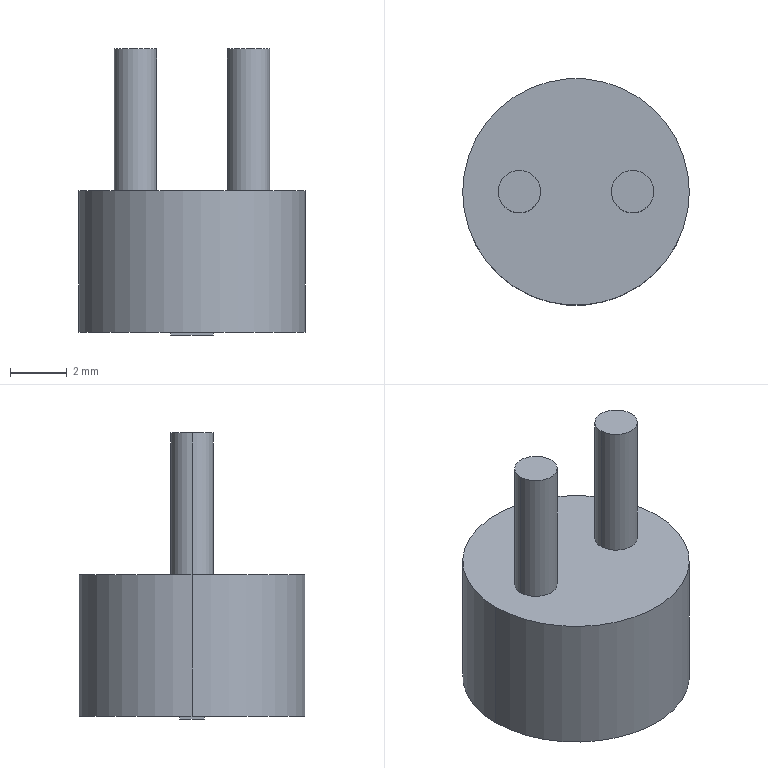Part | STEP file | 332 | 1 solid | 15 faces | box 8 x 8 x 10.1 mm | volume 269.13 mm3 | plane 9 | cylinder 6 | commonest cylinder face diameters 1.5 x4 8 x2
STEP:
#1=CARTESIAN_POINT('',(0.,0.,0.));
#2=DIRECTION('',(0.,0.,1.));
#3=DIRECTION('',(1.,0.,0.));
#4=AXIS2_PLACEMENT_3D('',#1,#2,#3);
#5=CARTESIAN_POINT('',(2.75,0.,10.));
#6=VERTEX_POINT('',#5);
#7=CARTESIAN_POINT('',(1.25,0.,10.));
#8=VERTEX_POINT('',#7);
#9=CARTESIAN_POINT('',(2.,0.,10.));
#10=DIRECTION('',(0.,0.,1.));
#11=DIRECTION('',(-1.,0.,0.));
#12=AXIS2_PLACEMENT_3D('',#9,#10,#11);
#13=CIRCLE('',#12,0.75);
#14=CARTESIAN_POINT('',(2.,0.,10.));
#15=DIRECTION('',(0.,0.,-1.));
#16=DIRECTION('',(-1.,0.,0.));
#17=AXIS2_PLACEMENT_3D('',#14,#15,#16);
#18=CYLINDRICAL_SURFACE('',#17,0.75);
#19=CARTESIAN_POINT('',(6.283,0.));
#20=DIRECTION('',(-1.,0.));
#21=VECTOR('',#20,1.);
#22=LINE('',#19,#21);
#23=(GEOMETRIC_REPRESENTATION_CONTEXT(2)PARAMETRIC_REPRESENTATION_CONTEXT()REPRESENTATION_CONTEXT('',''));
#24=DEFINITIONAL_REPRESENTATION('',(#22),#23);
#25=PCURVE('',#18,#24);
#26=CARTESIAN_POINT('',(2.,0.,10.));
#27=DIRECTION('',(0.,0.,-1.));
#28=DIRECTION('',(-1.,0.,0.));
#29=AXIS2_PLACEMENT_3D('',#26,#27,#28);
#30=PLANE('',#29);
#31=CARTESIAN_POINT('',(0.75,0.));
#32=CARTESIAN_POINT('',(0.75,-1.299));
#33=CARTESIAN_POINT('',(-0.375,-0.6495));
#34=CARTESIAN_POINT('',(-1.5,0.));
#35=CARTESIAN_POINT('',(-0.375,0.6495));
#36=CARTESIAN_POINT('',(0.75,1.299));
#37=CARTESIAN_POINT('',(0.75,0.));
#38=(BOUNDED_CURVE()B_SPLINE_CURVE(2,(#31,#32,#33,#34,#35,#36,#37),.UNSPECIFIED.,.T.,.F.)B_SPLINE_CURVE_WITH_KNOTS((1,2,2,2,2,1),(-2.094,0.,2.094,4.189,6.283,8.378),.UNSPECIFIED.)CURVE()GEOMETRIC_REPRESENTATION_ITEM()RATIONAL_B_SPLINE_CURVE((1.,0.5,1.,0.5,1.,0.5,1.))REPRESENTATION_ITEM(''));
#39=(GEOMETRIC_REPRESENTATION_CONTEXT(2)PARAMETRIC_REPRESENTATION_CONTEXT()REPRESENTATION_CONTEXT('',''));
#40=DEFINITIONAL_REPRESENTATION('',(#38),#39);
#41=PCURVE('',#30,#40);
#42=SURFACE_CURVE('',#13,(#25,#41),.PCURVE_S1.);
#43=EDGE_CURVE('',#6,#8,#42,.T.);
#44=ORIENTED_EDGE('',*,*,#43,.F.);
#45=CARTESIAN_POINT('',(2.75,0.,5.));
#46=VERTEX_POINT('',#45);
#47=CARTESIAN_POINT('',(2.75,0.,10.));
#48=DIRECTION('',(0.,0.,-1.));
#49=VECTOR('',#48,1.);
#50=LINE('',#47,#49);
#51=CARTESIAN_POINT('',(3.142,0.));
#52=DIRECTION('',(0.,1.));
#53=VECTOR('',#52,1.);
#54=LINE('',#51,#53);
#55=(GEOMETRIC_REPRESENTATION_CONTEXT(2)PARAMETRIC_REPRESENTATION_CONTEXT()REPRESENTATION_CONTEXT('',''));
#56=DEFINITIONAL_REPRESENTATION('',(#54),#55);
#57=PCURVE('',#18,#56);
#58=CARTESIAN_POINT('',(2.,0.,10.));
#59=DIRECTION('',(0.,0.,-1.));
#60=DIRECTION('',(-1.,0.,0.));
#61=AXIS2_PLACEMENT_3D('',#58,#59,#60);
#62=CYLINDRICAL_SURFACE('',#61,0.75);
#63=CARTESIAN_POINT('',(3.142,0.));
#64=DIRECTION('',(0.,1.));
#65=VECTOR('',#64,1.);
#66=LINE('',#63,#65);
#67=(GEOMETRIC_REPRESENTATION_CONTEXT(2)PARAMETRIC_REPRESENTATION_CONTEXT()REPRESENTATION_CONTEXT('',''));
#68=DEFINITIONAL_REPRESENTATION('',(#66),#67);
#69=PCURVE('',#62,#68);
#70=SURFACE_CURVE('',#50,(#57,#69),.PCURVE_S1.);
#71=EDGE_CURVE('',#6,#46,#70,.T.);
#72=ORIENTED_EDGE('',*,*,#71,.T.);
#73=CARTESIAN_POINT('',(1.25,0.,5.));
#74=VERTEX_POINT('',#73);
#75=CARTESIAN_POINT('',(2.,0.,5.));
#76=DIRECTION('',(0.,0.,1.));
#77=DIRECTION('',(-1.,0.,0.));
#78=AXIS2_PLACEMENT_3D('',#75,#76,#77);
#79=CIRCLE('',#78,0.75);
#80=CARTESIAN_POINT('',(6.283,5.));
#81=DIRECTION('',(-1.,0.));
#82=VECTOR('',#81,1.);
#83=LINE('',#80,#82);
#84=(GEOMETRIC_REPRESENTATION_CONTEXT(2)PARAMETRIC_REPRESENTATION_CONTEXT()REPRESENTATION_CONTEXT('',''));
#85=DEFINITIONAL_REPRESENTATION('',(#83),#84);
#86=PCURVE('',#18,#85);
#87=CARTESIAN_POINT('',(0.,0.,5.));
#88=DIRECTION('',(0.,0.,1.));
#89=DIRECTION('',(1.,0.,0.));
#90=AXIS2_PLACEMENT_3D('',#87,#88,#89);
#91=PLANE('',#90);
#92=CARTESIAN_POINT('',(2.,0.));
#93=DIRECTION('',(-1.,0.));
#94=AXIS2_PLACEMENT_2D('',#92,#93);
#95=CIRCLE('',#94,0.75);
#96=(GEOMETRIC_REPRESENTATION_CONTEXT(2)PARAMETRIC_REPRESENTATION_CONTEXT()REPRESENTATION_CONTEXT('',''));
#97=DEFINITIONAL_REPRESENTATION('',(#95),#96);
#98=PCURVE('',#91,#97);
#99=SURFACE_CURVE('',#79,(#86,#98),.PCURVE_S1.);
#100=EDGE_CURVE('',#46,#74,#99,.T.);
#101=ORIENTED_EDGE('',*,*,#100,.T.);
#102=CARTESIAN_POINT('',(1.25,0.,10.));
#103=DIRECTION('',(0.,0.,-1.));
#104=VECTOR('',#103,1.);
#105=LINE('',#102,#104);
#106=CARTESIAN_POINT('',(0.,0.));
#107=DIRECTION('',(0.,1.));
#108=VECTOR('',#107,1.);
#109=LINE('',#106,#108);
#110=(GEOMETRIC_REPRESENTATION_CONTEXT(2)PARAMETRIC_REPRESENTATION_CONTEXT()REPRESENTATION_CONTEXT('',''));
#111=DEFINITIONAL_REPRESENTATION('',(#109),#110);
#112=PCURVE('',#18,#111);
#113=CARTESIAN_POINT('',(6.283,0.));
#114=DIRECTION('',(0.,1.));
#115=VECTOR('',#114,1.);
#116=LINE('',#113,#115);
#117=(GEOMETRIC_REPRESENTATION_CONTEXT(2)PARAMETRIC_REPRESENTATION_CONTEXT()REPRESENTATION_CONTEXT('',''));
#118=DEFINITIONAL_REPRESENTATION('',(#116),#117);
#119=PCURVE('',#62,#118);
#120=SURFACE_CURVE('',#105,(#112,#119),.PCURVE_S1.);
#121=EDGE_CURVE('',#8,#74,#120,.T.);
#122=ORIENTED_EDGE('',*,*,#121,.F.);
#123=EDGE_LOOP('',(#44,#72,#101,#122));
#124=FACE_BOUND('',#123,.T.);
#125=ADVANCED_FACE('',(#124),#18,.T.);
#126=CARTESIAN_POINT('',(-1.25,0.,10.));
#127=VERTEX_POINT('',#126);
#128=CARTESIAN_POINT('',(-2.75,0.,10.));
#129=VERTEX_POINT('',#128);
#130=CARTESIAN_POINT('',(-2.,0.,10.));
#131=DIRECTION('',(0.,0.,1.));
#132=DIRECTION('',(1.,0.,0.));
#133=AXIS2_PLACEMENT_3D('',#130,#131,#132);
#134=CIRCLE('',#133,0.75);
#135=CARTESIAN_POINT('',(-2.,0.,10.));
#136=DIRECTION('',(0.,0.,-1.));
#137=DIRECTION('',(-1.,0.,0.));
#138=AXIS2_PLACEMENT_3D('',#135,#136,#137);
#139=CYLINDRICAL_SURFACE('',#138,0.75);
#140=CARTESIAN_POINT('',(3.142,0.));
#141=DIRECTION('',(-1.,0.));
#142=VECTOR('',#141,1.);
#143=LINE('',#140,#142);
#144=(GEOMETRIC_REPRESENTATION_CONTEXT(2)PARAMETRIC_REPRESENTATION_CONTEXT()REPRESENTATION_CONTEXT('',''));
#145=DEFINITIONAL_REPRESENTATION('',(#143),#144);
#146=PCURVE('',#139,#145);
#147=CARTESIAN_POINT('',(-2.,0.,10.));
#148=DIRECTION('',(0.,0.,1.));
#149=DIRECTION('',(1.,0.,0.));
#150=AXIS2_PLACEMENT_3D('',#147,#148,#149);
#151=PLANE('',#150);
#152=CARTESIAN_POINT('',(0.,0.));
#153=DIRECTION('',(1.,0.));
#154=AXIS2_PLACEMENT_2D('',#152,#153);
#155=CIRCLE('',#154,0.75);
#156=(GEOMETRIC_REPRESENTATION_CONTEXT(2)PARAMETRIC_REPRESENTATION_CONTEXT()REPRESENTATION_CONTEXT('',''));
#157=DEFINITIONAL_REPRESENTATION('',(#155),#156);
#158=PCURVE('',#151,#157);
#159=SURFACE_CURVE('',#134,(#146,#158),.PCURVE_S1.);
#160=EDGE_CURVE('',#127,#129,#159,.T.);
#161=ORIENTED_EDGE('',*,*,#160,.F.);
#162=CARTESIAN_POINT('',(-1.25,0.,5.));
#163=VERTEX_POINT('',#162);
#164=CARTESIAN_POINT('',(-1.25,0.,10.));
#165=DIRECTION('',(0.,0.,-1.));
#166=VECTOR('',#165,1.);
#167=LINE('',#164,#166);
#168=CARTESIAN_POINT('',(3.142,0.));
#169=DIRECTION('',(0.,1.));
#170=VECTOR('',#169,1.);
#171=LINE('',#168,#170);
#172=(GEOMETRIC_REPRESENTATION_CONTEXT(2)PARAMETRIC_REPRESENTATION_CONTEXT()REPRESENTATION_CONTEXT('',''));
#173=DEFINITIONAL_REPRESENTATION('',(#171),#172);
#174=PCURVE('',#139,#173);
#175=CARTESIAN_POINT('',(-2.,0.,10.));
#176=DIRECTION('',(0.,0.,-1.));
#177=DIRECTION('',(-1.,0.,0.));
#178=AXIS2_PLACEMENT_3D('',#175,#176,#177);
#179=CYLINDRICAL_SURFACE('',#178,0.75);
#180=CARTESIAN_POINT('',(3.142,0.));
#181=DIRECTION('',(0.,1.));
#182=VECTOR('',#181,1.);
#183=LINE('',#180,#182);
#184=(GEOMETRIC_REPRESENTATION_CONTEXT(2)PARAMETRIC_REPRESENTATION_CONTEXT()REPRESENTATION_CONTEXT('',''));
#185=DEFINITIONAL_REPRESENTATION('',(#183),#184);
#186=PCURVE('',#179,#185);
#187=SURFACE_CURVE('',#167,(#174,#186),.PCURVE_S1.);
#188=EDGE_CURVE('',#127,#163,#187,.T.);
#189=ORIENTED_EDGE('',*,*,#188,.T.);
#190=CARTESIAN_POINT('',(-2.75,0.,5.));
#191=VERTEX_POINT('',#190);
#192=CARTESIAN_POINT('',(-2.,0.,5.));
#193=DIRECTION('',(0.,0.,1.));
#194=DIRECTION('',(1.,0.,0.));
#195=AXIS2_PLACEMENT_3D('',#192,#193,#194);
#196=CIRCLE('',#195,0.75);
#197=CARTESIAN_POINT('',(3.142,5.));
#198=DIRECTION('',(-1.,0.));
#199=VECTOR('',#198,1.);
#200=LINE('',#197,#199);
#201=(GEOMETRIC_REPRESENTATION_CONTEXT(2)PARAMETRIC_REPRESENTATION_CONTEXT()REPRESENTATION_CONTEXT('',''));
#202=DEFINITIONAL_REPRESENTATION('',(#200),#201);
#203=PCURVE('',#139,#202);
#204=CARTESIAN_POINT('',(-2.,0.));
#205=DIRECTION('',(1.,0.));
#206=AXIS2_PLACEMENT_2D('',#204,#205);
#207=CIRCLE('',#206,0.75);
#208=(GEOMETRIC_REPRESENTATION_CONTEXT(2)PARAMETRIC_REPRESENTATION_CONTEXT()REPRESENTATION_CONTEXT('',''));
#209=DEFINITIONAL_REPRESENTATION('',(#207),#208);
#210=PCURVE('',#91,#209);
#211=SURFACE_CURVE('',#196,(#203,#210),.PCURVE_S1.);
#212=EDGE_CURVE('',#163,#191,#211,.T.);
#213=ORIENTED_EDGE('',*,*,#212,.T.);
#214=CARTESIAN_POINT('',(-2.75,0.,10.));
#215=DIRECTION('',(0.,0.,-1.));
#216=VECTOR('',#215,1.);
#217=LINE('',#214,#216);
#218=CARTESIAN_POINT('',(0.,0.));
#219=DIRECTION('',(0.,1.));
#220=VECTOR('',#219,1.);
#221=LINE('',#218,#220);
#222=(GEOMETRIC_REPRESENTATION_CONTEXT(2)PARAMETRIC_REPRESENTATION_CONTEXT()REPRESENTATION_CONTEXT('',''));
#223=DEFINITIONAL_REPRESENTATION('',(#221),#222);
#224=PCURVE('',#139,#223);
#225=CARTESIAN_POINT('',(6.283,0.));
#226=DIRECTION('',(0.,1.));
#227=VECTOR('',#226,1.);
#228=LINE('',#225,#227);
#229=(GEOMETRIC_REPRESENTATION_CONTEXT(2)PARAMETRIC_REPRESENTATION_CONTEXT()REPRESENTATION_CONTEXT('',''));
#230=DEFINITIONAL_REPRESENTATION('',(#228),#229);
#231=PCURVE('',#179,#230);
#232=SURFACE_CURVE('',#217,(#224,#231),.PCURVE_S1.);
#233=EDGE_CURVE('',#129,#191,#232,.T.);
#234=ORIENTED_EDGE('',*,*,#233,.F.);
#235=EDGE_LOOP('',(#161,#189,#213,#234));
#236=FACE_BOUND('',#235,.T.);
#237=ADVANCED_FACE('',(#236),#139,.T.);
#238=CARTESIAN_POINT('',(4.,0.,5.));
#239=VERTEX_POINT('',#238);
#240=CARTESIAN_POINT('',(-4.,0.,5.));
#241=VERTEX_POINT('',#240);
#242=CARTESIAN_POINT('',(0.,0.,5.));
#243=DIRECTION('',(0.,0.,1.));
#244=DIRECTION('',(1.,0.,0.));
#245=AXIS2_PLACEMENT_3D('',#242,#243,#244);
#246=CIRCLE('',#245,4.);
#247=CARTESIAN_POINT('',(0.,0.,5.));
#248=DIRECTION('',(0.,0.,-1.));
#249=DIRECTION('',(-1.,0.,0.));
#250=AXIS2_PLACEMENT_3D('',#247,#248,#249);
#251=CYLINDRICAL_SURFACE('',#250,4.);
#252=CARTESIAN_POINT('',(3.142,0.));
#253=DIRECTION('',(-1.,0.));
#254=VECTOR('',#253,1.);
#255=LINE('',#252,#254);
#256=(GEOMETRIC_REPRESENTATION_CONTEXT(2)PARAMETRIC_REPRESENTATION_CONTEXT()REPRESENTATION_CONTEXT('',''));
#257=DEFINITIONAL_REPRESENTATION('',(#255),#256);
#258=PCURVE('',#251,#257);
#259=CARTESIAN_POINT('',(0.,0.));
#260=DIRECTION('',(1.,0.));
#261=AXIS2_PLACEMENT_2D('',#259,#260);
#262=CIRCLE('',#261,4.);
#263=(GEOMETRIC_REPRESENTATION_CONTEXT(2)PARAMETRIC_REPRESENTATION_CONTEXT()REPRESENTATION_CONTEXT('',''));
#264=DEFINITIONAL_REPRESENTATION('',(#262),#263);
#265=PCURVE('',#91,#264);
#266=SURFACE_CURVE('',#246,(#258,#265),.PCURVE_S1.);
#267=EDGE_CURVE('',#239,#241,#266,.T.);
#268=ORIENTED_EDGE('',*,*,#267,.F.);
#269=CARTESIAN_POINT('',(4.,0.,0.));
#270=VERTEX_POINT('',#269);
#271=CARTESIAN_POINT('',(4.,0.,5.));
#272=DIRECTION('',(0.,0.,-1.));
#273=VECTOR('',#272,1.);
#274=LINE('',#271,#273);
#275=CARTESIAN_POINT('',(3.142,0.));
#276=DIRECTION('',(0.,1.));
#277=VECTOR('',#276,1.);
#278=LINE('',#275,#277);
#279=(GEOMETRIC_REPRESENTATION_CONTEXT(2)PARAMETRIC_REPRESENTATION_CONTEXT()REPRESENTATION_CONTEXT('',''));
#280=DEFINITIONAL_REPRESENTATION('',(#278),#279);
#281=PCURVE('',#251,#280);
#282=CARTESIAN_POINT('',(0.,0.,5.));
#283=DIRECTION('',(0.,0.,-1.));
#284=DIRECTION('',(-1.,0.,0.));
#285=AXIS2_PLACEMENT_3D('',#282,#283,#284);
#286=CYLINDRICAL_SURFACE('',#285,4.);
#287=CARTESIAN_POINT('',(3.142,0.));
#288=DIRECTION('',(0.,1.));
#289=VECTOR('',#288,1.);
#290=LINE('',#287,#289);
#291=(GEOMETRIC_REPRESENTATION_CONTEXT(2)PARAMETRIC_REPRESENTATION_CONTEXT()REPRESENTATION_CONTEXT('',''));
#292=DEFINITIONAL_REPRESENTATION('',(#290),#291);
#293=PCURVE('',#286,#292);
#294=SURFACE_CURVE('',#274,(#281,#293),.PCURVE_S1.);
#295=EDGE_CURVE('',#239,#270,#294,.T.);
#296=ORIENTED_EDGE('',*,*,#295,.T.);
#297=CARTESIAN_POINT('',(-4.,0.,0.));
#298=VERTEX_POINT('',#297);
#299=CARTESIAN_POINT('',(0.,0.,0.));
#300=DIRECTION('',(0.,0.,1.));
#301=DIRECTION('',(1.,0.,0.));
#302=AXIS2_PLACEMENT_3D('',#299,#300,#301);
#303=CIRCLE('',#302,4.);
#304=CARTESIAN_POINT('',(3.142,5.));
#305=DIRECTION('',(-1.,0.));
#306=VECTOR('',#305,1.);
#307=LINE('',#304,#306);
#308=(GEOMETRIC_REPRESENTATION_CONTEXT(2)PARAMETRIC_REPRESENTATION_CONTEXT()REPRESENTATION_CONTEXT('',''));
#309=DEFINITIONAL_REPRESENTATION('',(#307),#308);
#310=PCURVE('',#251,#309);
#311=CARTESIAN_POINT('',(0.,0.,0.));
#312=DIRECTION('',(0.,0.,1.));
#313=DIRECTION('',(1.,0.,0.));
#314=AXIS2_PLACEMENT_3D('',#311,#312,#313);
#315=PLANE('',#314);
#316=CARTESIAN_POINT('',(0.,0.));
#317=DIRECTION('',(1.,0.));
#318=AXIS2_PLACEMENT_2D('',#316,#317);
#319=CIRCLE('',#318,4.);
#320=(GEOMETRIC_REPRESENTATION_CONTEXT(2)PARAMETRIC_REPRESENTATION_CONTEXT()REPRESENTATION_CONTEXT('',''));
#321=DEFINITIONAL_REPRESENTATION('',(#319),#320);
#322=PCURVE('',#315,#321);
#323=SURFACE_CURVE('',#303,(#310,#322),.PCURVE_S1.);
#324=EDGE_CURVE('',#270,#298,#323,.T.);
#325=ORIENTED_EDGE('',*,*,#324,.T.);
#326=CARTESIAN_POINT('',(-4.,0.,5.));
#327=DIRECTION('',(0.,0.,-1.));
#328=VECTOR('',#327,1.);
#329=LINE('',#326,#328);
#330=CARTESIAN_POINT('',(0.,0.));
#331=DIRECTION('',(0.,1.));
#332=VECTOR('',#331,1.);
#333=LINE('',#330,#332);
#334=(GEOMETRIC_REPRESENTATION_CONTEXT(2)PARAMETRIC_REPRESENTATION_CONTEXT()REPRESENTATION_CONTEXT('',''));
#335=DEFINITIONAL_REPRESENTATION('',(#333),#334);
#336=PCURVE('',#251,#335);
#337=CARTESIAN_POINT('',(6.283,0.));
#338=DIRECTION('',(0.,1.));
#339=VECTOR('',#338,1.);
#340=LINE('',#337,#339);
#341=(GEOMETRIC_REPRESENTATION_CONTEXT(2)PARAMETRIC_REPRESENTATION_CONTEXT()REPRESENTATION_CONTEXT('',''));
#342=DEFINITIONAL_REPRESENTATION('',(#340),#341);
#343=PCURVE('',#286,#342);
#344=SURFACE_CURVE('',#329,(#336,#343),.PCURVE_S1.);
#345=EDGE_CURVE('',#241,#298,#344,.T.);
#346=ORIENTED_EDGE('',*,*,#345,.F.);
#347=EDGE_LOOP('',(#268,#296,#325,#346));
#348=FACE_BOUND('',#347,.T.);
#349=ADVANCED_FACE('',(#348),#251,.T.);
#350=CARTESIAN_POINT('',(0.,0.,0.));
#351=DIRECTION('',(0.,0.,1.));
#352=DIRECTION('',(1.,0.,0.));
#353=AXIS2_PLACEMENT_3D('',#350,#351,#352);
#354=CIRCLE('',#353,4.);
#355=CARTESIAN_POINT('',(0.,0.));
#356=DIRECTION('',(1.,0.));
#357=AXIS2_PLACEMENT_2D('',#355,#356);
#358=CIRCLE('',#357,4.);
#359=(GEOMETRIC_REPRESENTATION_CONTEXT(2)PARAMETRIC_REPRESENTATION_CONTEXT()REPRESENTATION_CONTEXT('',''));
#360=DEFINITIONAL_REPRESENTATION('',(#358),#359);
#361=PCURVE('',#315,#360);
#362=CARTESIAN_POINT('',(9.425,5.));
#363=DIRECTION('',(-1.,0.));
#364=VECTOR('',#363,1.);
#365=LINE('',#362,#364);
#366=(GEOMETRIC_REPRESENTATION_CONTEXT(2)PARAMETRIC_REPRESENTATION_CONTEXT()REPRESENTATION_CONTEXT('',''));
#367=DEFINITIONAL_REPRESENTATION('',(#365),#366);
#368=PCURVE('',#286,#367);
#369=SURFACE_CURVE('',#354,(#361,#368),.PCURVE_S1.);
#370=EDGE_CURVE('',#298,#270,#369,.T.);
#371=ORIENTED_EDGE('',*,*,#370,.F.);
#372=ORIENTED_EDGE('',*,*,#324,.F.);
#373=EDGE_LOOP('',(#371,#372));
#374=FACE_BOUND('',#373,.T.);
#375=CARTESIAN_POINT('',(0.7479,0.4396,0.));
#376=VERTEX_POINT('',#375);
#377=CARTESIAN_POINT('',(0.7479,-0.4396,0.));
#378=VERTEX_POINT('',#377);
#379=CARTESIAN_POINT('',(0.7479,0.4396,0.));
#380=DIRECTION('',(0.,-1.,0.));
#381=VECTOR('',#380,1.);
#382=LINE('',#379,#381);
#383=CARTESIAN_POINT('',(0.7479,0.4396));
#384=DIRECTION('',(0.,-1.));
#385=VECTOR('',#384,1.);
#386=LINE('',#383,#385);
#387=(GEOMETRIC_REPRESENTATION_CONTEXT(2)PARAMETRIC_REPRESENTATION_CONTEXT()REPRESENTATION_CONTEXT('',''));
#388=DEFINITIONAL_REPRESENTATION('',(#386),#387);
#389=PCURVE('',#315,#388);
#390=CARTESIAN_POINT('',(0.7479,0.4396,-0.1));
#391=DIRECTION('',(-1.,0.,0.));
#392=DIRECTION('',(0.,0.,1.));
#393=AXIS2_PLACEMENT_3D('',#390,#391,#392);
#394=PLANE('',#393);
#395=CARTESIAN_POINT('',(0.1,0.));
#396=DIRECTION('',(0.,-1.));
#397=VECTOR('',#396,1.);
#398=LINE('',#395,#397);
#399=(GEOMETRIC_REPRESENTATION_CONTEXT(2)PARAMETRIC_REPRESENTATION_CONTEXT()REPRESENTATION_CONTEXT('',''));
#400=DEFINITIONAL_REPRESENTATION('',(#398),#399);
#401=PCURVE('',#394,#400);
#402=SURFACE_CURVE('',#382,(#389,#401),.PCURVE_S1.);
#403=EDGE_CURVE('',#376,#378,#402,.T.);
#404=ORIENTED_EDGE('',*,*,#403,.F.);
#405=CARTESIAN_POINT('',(-0.7479,0.4396,0.));
#406=VERTEX_POINT('',#405);
#407=CARTESIAN_POINT('',(-0.7479,0.4396,0.));
#408=DIRECTION('',(1.,0.,0.));
#409=VECTOR('',#408,1.);
#410=LINE('',#407,#409);
#411=CARTESIAN_POINT('',(-0.7479,0.4396));
#412=DIRECTION('',(1.,0.));
#413=VECTOR('',#412,1.);
#414=LINE('',#411,#413);
#415=(GEOMETRIC_REPRESENTATION_CONTEXT(2)PARAMETRIC_REPRESENTATION_CONTEXT()REPRESENTATION_CONTEXT('',''));
#416=DEFINITIONAL_REPRESENTATION('',(#414),#415);
#417=PCURVE('',#315,#416);
#418=CARTESIAN_POINT('',(-0.7479,0.4396,-0.1));
#419=DIRECTION('',(0.,-1.,0.));
#420=DIRECTION('',(0.,0.,-1.));
#421=AXIS2_PLACEMENT_3D('',#418,#419,#420);
#422=PLANE('',#421);
#423=CARTESIAN_POINT('',(-0.1,0.));
#424=DIRECTION('',(0.,1.));
#425=VECTOR('',#424,1.);
#426=LINE('',#423,#425);
#427=(GEOMETRIC_REPRESENTATION_CONTEXT(2)PARAMETRIC_REPRESENTATION_CONTEXT()REPRESENTATION_CONTEXT('',''));
#428=DEFINITIONAL_REPRESENTATION('',(#426),#427);
#429=PCURVE('',#422,#428);
#430=SURFACE_CURVE('',#410,(#417,#429),.PCURVE_S1.);
#431=EDGE_CURVE('',#406,#376,#430,.T.);
#432=ORIENTED_EDGE('',*,*,#431,.F.);
#433=CARTESIAN_POINT('',(-0.7479,-0.4396,0.));
#434=VERTEX_POINT('',#433);
#435=CARTESIAN_POINT('',(-0.7479,0.4396,0.));
#436=DIRECTION('',(0.,1.,0.));
#437=VECTOR('',#436,1.);
#438=LINE('',#435,#437);
#439=CARTESIAN_POINT('',(-0.7479,0.4396));
#440=DIRECTION('',(0.,1.));
#441=VECTOR('',#440,1.);
#442=LINE('',#439,#441);
#443=(GEOMETRIC_REPRESENTATION_CONTEXT(2)PARAMETRIC_REPRESENTATION_CONTEXT()REPRESENTATION_CONTEXT('',''));
#444=DEFINITIONAL_REPRESENTATION('',(#442),#443);
#445=PCURVE('',#315,#444);
#446=CARTESIAN_POINT('',(-0.7479,0.4396,-0.1));
#447=DIRECTION('',(1.,0.,0.));
#448=DIRECTION('',(0.,0.,-1.));
#449=AXIS2_PLACEMENT_3D('',#446,#447,#448);
#450=PLANE('',#449);
#451=CARTESIAN_POINT('',(-0.1,0.));
#452=DIRECTION('',(0.,1.));
#453=VECTOR('',#452,1.);
#454=LINE('',#451,#453);
#455=(GEOMETRIC_REPRESENTATION_CONTEXT(2)PARAMETRIC_REPRESENTATION_CONTEXT()REPRESENTATION_CONTEXT('',''));
#456=DEFINITIONAL_REPRESENTATION('',(#454),#455);
#457=PCURVE('',#450,#456);
#458=SURFACE_CURVE('',#438,(#445,#457),.PCURVE_S1.);
#459=EDGE_CURVE('',#434,#406,#458,.T.);
#460=ORIENTED_EDGE('',*,*,#459,.F.);
#461=CARTESIAN_POINT('',(-0.7479,-0.4396,0.));
#462=DIRECTION('',(-1.,0.,0.));
#463=VECTOR('',#462,1.);
#464=LINE('',#461,#463);
#465=CARTESIAN_POINT('',(-0.7479,-0.4396));
#466=DIRECTION('',(-1.,0.));
#467=VECTOR('',#466,1.);
#468=LINE('',#465,#467);
#469=(GEOMETRIC_REPRESENTATION_CONTEXT(2)PARAMETRIC_REPRESENTATION_CONTEXT()REPRESENTATION_CONTEXT('',''));
#470=DEFINITIONAL_REPRESENTATION('',(#468),#469);
#471=PCURVE('',#315,#470);
#472=CARTESIAN_POINT('',(-0.7479,-0.4396,-0.1));
#473=DIRECTION('',(0.,1.,0.));
#474=DIRECTION('',(0.,0.,1.));
#475=AXIS2_PLACEMENT_3D('',#472,#473,#474);
#476=PLANE('',#475);
#477=CARTESIAN_POINT('',(0.1,0.));
#478=DIRECTION('',(0.,-1.));
#479=VECTOR('',#478,1.);
#480=LINE('',#477,#479);
#481=(GEOMETRIC_REPRESENTATION_CONTEXT(2)PARAMETRIC_REPRESENTATION_CONTEXT()REPRESENTATION_CONTEXT('',''));
#482=DEFINITIONAL_REPRESENTATION('',(#480),#481);
#483=PCURVE('',#476,#482);
#484=SURFACE_CURVE('',#464,(#471,#483),.PCURVE_S1.);
#485=EDGE_CURVE('',#378,#434,#484,.T.);
#486=ORIENTED_EDGE('',*,*,#485,.F.);
#487=EDGE_LOOP('',(#404,#432,#460,#486));
#488=FACE_BOUND('',#487,.T.);
#489=ADVANCED_FACE('',(#374,#488),#315,.F.);
#490=CARTESIAN_POINT('',(-2.,0.,5.));
#491=DIRECTION('',(0.,0.,1.));
#492=DIRECTION('',(1.,0.,0.));
#493=AXIS2_PLACEMENT_3D('',#490,#491,#492);
#494=CIRCLE('',#493,0.75);
#495=CARTESIAN_POINT('',(-2.,0.));
#496=DIRECTION('',(1.,0.));
#497=AXIS2_PLACEMENT_2D('',#495,#496);
#498=CIRCLE('',#497,0.75);
#499=(GEOMETRIC_REPRESENTATION_CONTEXT(2)PARAMETRIC_REPRESENTATION_CONTEXT()REPRESENTATION_CONTEXT('',''));
#500=DEFINITIONAL_REPRESENTATION('',(#498),#499);
#501=PCURVE('',#91,#500);
#502=CARTESIAN_POINT('',(9.425,5.));
#503=DIRECTION('',(-1.,0.));
#504=VECTOR('',#503,1.);
#505=LINE('',#502,#504);
#506=(GEOMETRIC_REPRESENTATION_CONTEXT(2)PARAMETRIC_REPRESENTATION_CONTEXT()REPRESENTATION_CONTEXT('',''));
#507=DEFINITIONAL_REPRESENTATION('',(#505),#506);
#508=PCURVE('',#179,#507);
#509=SURFACE_CURVE('',#494,(#501,#508),.PCURVE_S1.);
#510=EDGE_CURVE('',#191,#163,#509,.T.);
#511=ORIENTED_EDGE('',*,*,#510,.F.);
#512=ORIENTED_EDGE('',*,*,#212,.F.);
#513=EDGE_LOOP('',(#511,#512));
#514=FACE_BOUND('',#513,.T.);
#515=CARTESIAN_POINT('',(0.,0.,5.));
#516=DIRECTION('',(0.,0.,1.));
#517=DIRECTION('',(1.,0.,0.));
#518=AXIS2_PLACEMENT_3D('',#515,#516,#517);
#519=CIRCLE('',#518,4.);
#520=CARTESIAN_POINT('',(0.,0.));
#521=DIRECTION('',(1.,0.));
#522=AXIS2_PLACEMENT_2D('',#520,#521);
#523=CIRCLE('',#522,4.);
#524=(GEOMETRIC_REPRESENTATION_CONTEXT(2)PARAMETRIC_REPRESENTATION_CONTEXT()REPRESENTATION_CONTEXT('',''));
#525=DEFINITIONAL_REPRESENTATION('',(#523),#524);
#526=PCURVE('',#91,#525);
#527=CARTESIAN_POINT('',(9.425,0.));
#528=DIRECTION('',(-1.,0.));
#529=VECTOR('',#528,1.);
#530=LINE('',#527,#529);
#531=(GEOMETRIC_REPRESENTATION_CONTEXT(2)PARAMETRIC_REPRESENTATION_CONTEXT()REPRESENTATION_CONTEXT('',''));
#532=DEFINITIONAL_REPRESENTATION('',(#530),#531);
#533=PCURVE('',#286,#532);
#534=SURFACE_CURVE('',#519,(#526,#533),.PCURVE_S1.);
#535=EDGE_CURVE('',#241,#239,#534,.T.);
#536=ORIENTED_EDGE('',*,*,#535,.T.);
#537=ORIENTED_EDGE('',*,*,#267,.T.);
#538=EDGE_LOOP('',(#536,#537));
#539=FACE_BOUND('',#538,.T.);
#540=CARTESIAN_POINT('',(2.,0.,5.));
#541=DIRECTION('',(0.,0.,1.));
#542=DIRECTION('',(-1.,0.,0.));
#543=AXIS2_PLACEMENT_3D('',#540,#541,#542);
#544=CIRCLE('',#543,0.75);
#545=CARTESIAN_POINT('',(2.,0.));
#546=DIRECTION('',(-1.,0.));
#547=AXIS2_PLACEMENT_2D('',#545,#546);
#548=CIRCLE('',#547,0.75);
#549=(GEOMETRIC_REPRESENTATION_CONTEXT(2)PARAMETRIC_REPRESENTATION_CONTEXT()REPRESENTATION_CONTEXT('',''));
#550=DEFINITIONAL_REPRESENTATION('',(#548),#549);
#551=PCURVE('',#91,#550);
#552=CARTESIAN_POINT('',(6.283,5.));
#553=DIRECTION('',(-1.,0.));
#554=VECTOR('',#553,1.);
#555=LINE('',#552,#554);
#556=(GEOMETRIC_REPRESENTATION_CONTEXT(2)PARAMETRIC_REPRESENTATION_CONTEXT()REPRESENTATION_CONTEXT('',''));
#557=DEFINITIONAL_REPRESENTATION('',(#555),#556);
#558=PCURVE('',#62,#557);
#559=SURFACE_CURVE('',#544,(#551,#558),.PCURVE_S1.);
#560=EDGE_CURVE('',#74,#46,#559,.T.);
#561=ORIENTED_EDGE('',*,*,#560,.F.);
#562=ORIENTED_EDGE('',*,*,#100,.F.);
#563=EDGE_LOOP('',(#561,#562));
#564=FACE_BOUND('',#563,.T.);
#565=ADVANCED_FACE('',(#514,#539,#564),#91,.T.);
#566=ORIENTED_EDGE('',*,*,#295,.F.);
#567=ORIENTED_EDGE('',*,*,#535,.F.);
#568=ORIENTED_EDGE('',*,*,#345,.T.);
#569=ORIENTED_EDGE('',*,*,#370,.T.);
#570=EDGE_LOOP('',(#566,#567,#568,#569));
#571=FACE_BOUND('',#570,.T.);
#572=ADVANCED_FACE('',(#571),#286,.T.);
#573=ORIENTED_EDGE('',*,*,#188,.F.);
#574=CARTESIAN_POINT('',(-2.,0.,10.));
#575=DIRECTION('',(0.,0.,1.));
#576=DIRECTION('',(1.,0.,0.));
#577=AXIS2_PLACEMENT_3D('',#574,#575,#576);
#578=CIRCLE('',#577,0.75);
#579=CARTESIAN_POINT('',(9.425,0.));
#580=DIRECTION('',(-1.,0.));
#581=VECTOR('',#580,1.);
#582=LINE('',#579,#581);
#583=(GEOMETRIC_REPRESENTATION_CONTEXT(2)PARAMETRIC_REPRESENTATION_CONTEXT()REPRESENTATION_CONTEXT('',''));
#584=DEFINITIONAL_REPRESENTATION('',(#582),#583);
#585=PCURVE('',#179,#584);
#586=CARTESIAN_POINT('',(0.,0.));
#587=DIRECTION('',(1.,0.));
#588=AXIS2_PLACEMENT_2D('',#586,#587);
#589=CIRCLE('',#588,0.75);
#590=(GEOMETRIC_REPRESENTATION_CONTEXT(2)PARAMETRIC_REPRESENTATION_CONTEXT()REPRESENTATION_CONTEXT('',''));
#591=DEFINITIONAL_REPRESENTATION('',(#589),#590);
#592=PCURVE('',#151,#591);
#593=SURFACE_CURVE('',#578,(#585,#592),.PCURVE_S1.);
#594=EDGE_CURVE('',#129,#127,#593,.T.);
#595=ORIENTED_EDGE('',*,*,#594,.F.);
#596=ORIENTED_EDGE('',*,*,#233,.T.);
#597=ORIENTED_EDGE('',*,*,#510,.T.);
#598=EDGE_LOOP('',(#573,#595,#596,#597));
#599=FACE_BOUND('',#598,.T.);
#600=ADVANCED_FACE('',(#599),#179,.T.);
#601=ORIENTED_EDGE('',*,*,#594,.T.);
#602=ORIENTED_EDGE('',*,*,#160,.T.);
#603=EDGE_LOOP('',(#601,#602));
#604=FACE_BOUND('',#603,.T.);
#605=ADVANCED_FACE('',(#604),#151,.T.);
#606=ORIENTED_EDGE('',*,*,#71,.F.);
#607=CARTESIAN_POINT('',(2.,0.,10.));
#608=DIRECTION('',(0.,0.,1.));
#609=DIRECTION('',(-1.,0.,0.));
#610=AXIS2_PLACEMENT_3D('',#607,#608,#609);
#611=CIRCLE('',#610,0.75);
#612=CARTESIAN_POINT('',(6.283,0.));
#613=DIRECTION('',(-1.,0.));
#614=VECTOR('',#613,1.);
#615=LINE('',#612,#614);
#616=(GEOMETRIC_REPRESENTATION_CONTEXT(2)PARAMETRIC_REPRESENTATION_CONTEXT()REPRESENTATION_CONTEXT('',''));
#617=DEFINITIONAL_REPRESENTATION('',(#615),#616);
#618=PCURVE('',#62,#617);
#619=CARTESIAN_POINT('',(0.75,0.));
#620=CARTESIAN_POINT('',(0.75,-1.299));
#621=CARTESIAN_POINT('',(-0.375,-0.6495));
#622=CARTESIAN_POINT('',(-1.5,0.));
#623=CARTESIAN_POINT('',(-0.375,0.6495));
#624=CARTESIAN_POINT('',(0.75,1.299));
#625=CARTESIAN_POINT('',(0.75,0.));
#626=(BOUNDED_CURVE()B_SPLINE_CURVE(2,(#619,#620,#621,#622,#623,#624,#625),.UNSPECIFIED.,.T.,.F.)B_SPLINE_CURVE_WITH_KNOTS((1,2,2,2,2,1),(-2.094,0.,2.094,4.189,6.283,8.378),.UNSPECIFIED.)CURVE()GEOMETRIC_REPRESENTATION_ITEM()RATIONAL_B_SPLINE_CURVE((1.,0.5,1.,0.5,1.,0.5,1.))REPRESENTATION_ITEM(''));
#627=(GEOMETRIC_REPRESENTATION_CONTEXT(2)PARAMETRIC_REPRESENTATION_CONTEXT()REPRESENTATION_CONTEXT('',''));
#628=DEFINITIONAL_REPRESENTATION('',(#626),#627);
#629=PCURVE('',#30,#628);
#630=SURFACE_CURVE('',#611,(#618,#629),.PCURVE_S1.);
#631=EDGE_CURVE('',#8,#6,#630,.T.);
#632=ORIENTED_EDGE('',*,*,#631,.F.);
#633=ORIENTED_EDGE('',*,*,#121,.T.);
#634=ORIENTED_EDGE('',*,*,#560,.T.);
#635=EDGE_LOOP('',(#606,#632,#633,#634));
#636=FACE_BOUND('',#635,.T.);
#637=ADVANCED_FACE('',(#636),#62,.T.);
#638=ORIENTED_EDGE('',*,*,#631,.T.);
#639=ORIENTED_EDGE('',*,*,#43,.T.);
#640=EDGE_LOOP('',(#638,#639));
#641=FACE_BOUND('',#640,.T.);
#642=ADVANCED_FACE('',(#641),#30,.F.);
#643=ORIENTED_EDGE('',*,*,#403,.T.);
#644=CARTESIAN_POINT('',(0.7479,-0.4396,-0.1));
#645=VERTEX_POINT('',#644);
#646=CARTESIAN_POINT('',(0.7479,-0.4396,-0.1));
#647=DIRECTION('',(0.,0.,1.));
#648=VECTOR('',#647,1.);
#649=LINE('',#646,#648);
#650=CARTESIAN_POINT('',(0.,-0.8792));
#651=DIRECTION('',(1.,0.));
#652=VECTOR('',#651,1.);
#653=LINE('',#650,#652);
#654=(GEOMETRIC_REPRESENTATION_CONTEXT(2)PARAMETRIC_REPRESENTATION_CONTEXT()REPRESENTATION_CONTEXT('',''));
#655=DEFINITIONAL_REPRESENTATION('',(#653),#654);
#656=PCURVE('',#394,#655);
#657=CARTESIAN_POINT('',(0.,1.496));
#658=DIRECTION('',(1.,0.));
#659=VECTOR('',#658,1.);
#660=LINE('',#657,#659);
#661=(GEOMETRIC_REPRESENTATION_CONTEXT(2)PARAMETRIC_REPRESENTATION_CONTEXT()REPRESENTATION_CONTEXT('',''));
#662=DEFINITIONAL_REPRESENTATION('',(#660),#661);
#663=PCURVE('',#476,#662);
#664=SURFACE_CURVE('',#649,(#656,#663),.PCURVE_S1.);
#665=EDGE_CURVE('',#645,#378,#664,.T.);
#666=ORIENTED_EDGE('',*,*,#665,.F.);
#667=CARTESIAN_POINT('',(0.7479,0.4396,-0.1));
#668=VERTEX_POINT('',#667);
#669=CARTESIAN_POINT('',(0.7479,0.4396,-0.1));
#670=DIRECTION('',(0.,-1.,0.));
#671=VECTOR('',#670,1.);
#672=LINE('',#669,#671);
#673=CARTESIAN_POINT('',(0.,0.));
#674=DIRECTION('',(0.,-1.));
#675=VECTOR('',#674,1.);
#676=LINE('',#673,#675);
#677=(GEOMETRIC_REPRESENTATION_CONTEXT(2)PARAMETRIC_REPRESENTATION_CONTEXT()REPRESENTATION_CONTEXT('',''));
#678=DEFINITIONAL_REPRESENTATION('',(#676),#677);
#679=PCURVE('',#394,#678);
#680=CARTESIAN_POINT('',(0.,0.,-0.1));
#681=DIRECTION('',(0.,0.,1.));
#682=DIRECTION('',(1.,0.,0.));
#683=AXIS2_PLACEMENT_3D('',#680,#681,#682);
#684=PLANE('',#683);
#685=CARTESIAN_POINT('',(0.7479,0.4396));
#686=DIRECTION('',(0.,-1.));
#687=VECTOR('',#686,1.);
#688=LINE('',#685,#687);
#689=(GEOMETRIC_REPRESENTATION_CONTEXT(2)PARAMETRIC_REPRESENTATION_CONTEXT()REPRESENTATION_CONTEXT('',''));
#690=DEFINITIONAL_REPRESENTATION('',(#688),#689);
#691=PCURVE('',#684,#690);
#692=SURFACE_CURVE('',#672,(#679,#691),.PCURVE_S1.);
#693=EDGE_CURVE('',#668,#645,#692,.T.);
#694=ORIENTED_EDGE('',*,*,#693,.F.);
#695=CARTESIAN_POINT('',(0.7479,0.4396,-0.1));
#696=DIRECTION('',(0.,0.,1.));
#697=VECTOR('',#696,1.);
#698=LINE('',#695,#697);
#699=CARTESIAN_POINT('',(0.,0.));
#700=DIRECTION('',(1.,0.));
#701=VECTOR('',#700,1.);
#702=LINE('',#699,#701);
#703=(GEOMETRIC_REPRESENTATION_CONTEXT(2)PARAMETRIC_REPRESENTATION_CONTEXT()REPRESENTATION_CONTEXT('',''));
#704=DEFINITIONAL_REPRESENTATION('',(#702),#703);
#705=PCURVE('',#394,#704);
#706=CARTESIAN_POINT('',(0.,1.496));
#707=DIRECTION('',(-1.,0.));
#708=VECTOR('',#707,1.);
#709=LINE('',#706,#708);
#710=(GEOMETRIC_REPRESENTATION_CONTEXT(2)PARAMETRIC_REPRESENTATION_CONTEXT()REPRESENTATION_CONTEXT('',''));
#711=DEFINITIONAL_REPRESENTATION('',(#709),#710);
#712=PCURVE('',#422,#711);
#713=SURFACE_CURVE('',#698,(#705,#712),.PCURVE_S1.);
#714=EDGE_CURVE('',#668,#376,#713,.T.);
#715=ORIENTED_EDGE('',*,*,#714,.T.);
#716=EDGE_LOOP('',(#643,#666,#694,#715));
#717=FACE_BOUND('',#716,.T.);
#718=ADVANCED_FACE('',(#717),#394,.F.);
#719=ORIENTED_EDGE('',*,*,#485,.T.);
#720=CARTESIAN_POINT('',(-0.7479,-0.4396,-0.1));
#721=VERTEX_POINT('',#720);
#722=CARTESIAN_POINT('',(-0.7479,-0.4396,-0.1));
#723=DIRECTION('',(0.,0.,1.));
#724=VECTOR('',#723,1.);
#725=LINE('',#722,#724);
#726=CARTESIAN_POINT('',(0.,0.));
#727=DIRECTION('',(1.,0.));
#728=VECTOR('',#727,1.);
#729=LINE('',#726,#728);
#730=(GEOMETRIC_REPRESENTATION_CONTEXT(2)PARAMETRIC_REPRESENTATION_CONTEXT()REPRESENTATION_CONTEXT('',''));
#731=DEFINITIONAL_REPRESENTATION('',(#729),#730);
#732=PCURVE('',#476,#731);
#733=CARTESIAN_POINT('',(0.,-0.8792));
#734=DIRECTION('',(-1.,0.));
#735=VECTOR('',#734,1.);
#736=LINE('',#733,#735);
#737=(GEOMETRIC_REPRESENTATION_CONTEXT(2)PARAMETRIC_REPRESENTATION_CONTEXT()REPRESENTATION_CONTEXT('',''));
#738=DEFINITIONAL_REPRESENTATION('',(#736),#737);
#739=PCURVE('',#450,#738);
#740=SURFACE_CURVE('',#725,(#732,#739),.PCURVE_S1.);
#741=EDGE_CURVE('',#721,#434,#740,.T.);
#742=ORIENTED_EDGE('',*,*,#741,.F.);
#743=CARTESIAN_POINT('',(-0.7479,-0.4396,-0.1));
#744=DIRECTION('',(-1.,0.,0.));
#745=VECTOR('',#744,1.);
#746=LINE('',#743,#745);
#747=CARTESIAN_POINT('',(0.,0.));
#748=DIRECTION('',(0.,-1.));
#749=VECTOR('',#748,1.);
#750=LINE('',#747,#749);
#751=(GEOMETRIC_REPRESENTATION_CONTEXT(2)PARAMETRIC_REPRESENTATION_CONTEXT()REPRESENTATION_CONTEXT('',''));
#752=DEFINITIONAL_REPRESENTATION('',(#750),#751);
#753=PCURVE('',#476,#752);
#754=CARTESIAN_POINT('',(-0.7479,-0.4396));
#755=DIRECTION('',(-1.,0.));
#756=VECTOR('',#755,1.);
#757=LINE('',#754,#756);
#758=(GEOMETRIC_REPRESENTATION_CONTEXT(2)PARAMETRIC_REPRESENTATION_CONTEXT()REPRESENTATION_CONTEXT('',''));
#759=DEFINITIONAL_REPRESENTATION('',(#757),#758);
#760=PCURVE('',#684,#759);
#761=SURFACE_CURVE('',#746,(#753,#760),.PCURVE_S1.);
#762=EDGE_CURVE('',#645,#721,#761,.T.);
#763=ORIENTED_EDGE('',*,*,#762,.F.);
#764=ORIENTED_EDGE('',*,*,#665,.T.);
#765=EDGE_LOOP('',(#719,#742,#763,#764));
#766=FACE_BOUND('',#765,.T.);
#767=ADVANCED_FACE('',(#766),#476,.F.);
#768=ORIENTED_EDGE('',*,*,#459,.T.);
#769=CARTESIAN_POINT('',(-0.7479,0.4396,-0.1));
#770=VERTEX_POINT('',#769);
#771=CARTESIAN_POINT('',(-0.7479,0.4396,-0.1));
#772=DIRECTION('',(0.,0.,1.));
#773=VECTOR('',#772,1.);
#774=LINE('',#771,#773);
#775=CARTESIAN_POINT('',(0.,0.));
#776=DIRECTION('',(-1.,0.));
#777=VECTOR('',#776,1.);
#778=LINE('',#775,#777);
#779=(GEOMETRIC_REPRESENTATION_CONTEXT(2)PARAMETRIC_REPRESENTATION_CONTEXT()REPRESENTATION_CONTEXT('',''));
#780=DEFINITIONAL_REPRESENTATION('',(#778),#779);
#781=PCURVE('',#450,#780);
#782=CARTESIAN_POINT('',(0.,0.));
#783=DIRECTION('',(-1.,0.));
#784=VECTOR('',#783,1.);
#785=LINE('',#782,#784);
#786=(GEOMETRIC_REPRESENTATION_CONTEXT(2)PARAMETRIC_REPRESENTATION_CONTEXT()REPRESENTATION_CONTEXT('',''));
#787=DEFINITIONAL_REPRESENTATION('',(#785),#786);
#788=PCURVE('',#422,#787);
#789=SURFACE_CURVE('',#774,(#781,#788),.PCURVE_S1.);
#790=EDGE_CURVE('',#770,#406,#789,.T.);
#791=ORIENTED_EDGE('',*,*,#790,.F.);
#792=CARTESIAN_POINT('',(-0.7479,0.4396,-0.1));
#793=DIRECTION('',(0.,1.,0.));
#794=VECTOR('',#793,1.);
#795=LINE('',#792,#794);
#796=CARTESIAN_POINT('',(0.,0.));
#797=DIRECTION('',(0.,1.));
#798=VECTOR('',#797,1.);
#799=LINE('',#796,#798);
#800=(GEOMETRIC_REPRESENTATION_CONTEXT(2)PARAMETRIC_REPRESENTATION_CONTEXT()REPRESENTATION_CONTEXT('',''));
#801=DEFINITIONAL_REPRESENTATION('',(#799),#800);
#802=PCURVE('',#450,#801);
#803=CARTESIAN_POINT('',(-0.7479,0.4396));
#804=DIRECTION('',(0.,1.));
#805=VECTOR('',#804,1.);
#806=LINE('',#803,#805);
#807=(GEOMETRIC_REPRESENTATION_CONTEXT(2)PARAMETRIC_REPRESENTATION_CONTEXT()REPRESENTATION_CONTEXT('',''));
#808=DEFINITIONAL_REPRESENTATION('',(#806),#807);
#809=PCURVE('',#684,#808);
#810=SURFACE_CURVE('',#795,(#802,#809),.PCURVE_S1.);
#811=EDGE_CURVE('',#721,#770,#810,.T.);
#812=ORIENTED_EDGE('',*,*,#811,.F.);
#813=ORIENTED_EDGE('',*,*,#741,.T.);
#814=EDGE_LOOP('',(#768,#791,#812,#813));
#815=FACE_BOUND('',#814,.T.);
#816=ADVANCED_FACE('',(#815),#450,.F.);
#817=ORIENTED_EDGE('',*,*,#431,.T.);
#818=ORIENTED_EDGE('',*,*,#714,.F.);
#819=CARTESIAN_POINT('',(-0.7479,0.4396,-0.1));
#820=DIRECTION('',(1.,0.,0.));
#821=VECTOR('',#820,1.);
#822=LINE('',#819,#821);
#823=CARTESIAN_POINT('',(0.,0.));
#824=DIRECTION('',(0.,1.));
#825=VECTOR('',#824,1.);
#826=LINE('',#823,#825);
#827=(GEOMETRIC_REPRESENTATION_CONTEXT(2)PARAMETRIC_REPRESENTATION_CONTEXT()REPRESENTATION_CONTEXT('',''));
#828=DEFINITIONAL_REPRESENTATION('',(#826),#827);
#829=PCURVE('',#422,#828);
#830=CARTESIAN_POINT('',(-0.7479,0.4396));
#831=DIRECTION('',(1.,0.));
#832=VECTOR('',#831,1.);
#833=LINE('',#830,#832);
#834=(GEOMETRIC_REPRESENTATION_CONTEXT(2)PARAMETRIC_REPRESENTATION_CONTEXT()REPRESENTATION_CONTEXT('',''));
#835=DEFINITIONAL_REPRESENTATION('',(#833),#834);
#836=PCURVE('',#684,#835);
#837=SURFACE_CURVE('',#822,(#829,#836),.PCURVE_S1.);
#838=EDGE_CURVE('',#770,#668,#837,.T.);
#839=ORIENTED_EDGE('',*,*,#838,.F.);
#840=ORIENTED_EDGE('',*,*,#790,.T.);
#841=EDGE_LOOP('',(#817,#818,#839,#840));
#842=FACE_BOUND('',#841,.T.);
#843=ADVANCED_FACE('',(#842),#422,.F.);
#844=ORIENTED_EDGE('',*,*,#693,.T.);
#845=ORIENTED_EDGE('',*,*,#762,.T.);
#846=ORIENTED_EDGE('',*,*,#811,.T.);
#847=ORIENTED_EDGE('',*,*,#838,.T.);
#848=EDGE_LOOP('',(#844,#845,#846,#847));
#849=FACE_BOUND('',#848,.T.);
#850=ADVANCED_FACE('',(#849),#684,.F.);
#851=CLOSED_SHELL('',(#125,#237,#349,#489,#565,#572,#600,#605,#637,#642,#718,#767,#816,#843,#850));
#852=MANIFOLD_SOLID_BREP('',#851);
#853=(LENGTH_UNIT()NAMED_UNIT(*)SI_UNIT(.MILLI.,.METRE.));
#854=UNCERTAINTY_MEASURE_WITH_UNIT(LENGTH_MEASURE(0.0000001),#853,'','');
#855=(NAMED_UNIT(*)PLANE_ANGLE_UNIT()SI_UNIT($,.RADIAN.));
#856=(NAMED_UNIT(*)SI_UNIT($,.STERADIAN.)SOLID_ANGLE_UNIT());
#857=(GEOMETRIC_REPRESENTATION_CONTEXT(3)GLOBAL_UNCERTAINTY_ASSIGNED_CONTEXT((#854))GLOBAL_UNIT_ASSIGNED_CONTEXT((#853,#855,#856))REPRESENTATION_CONTEXT('',''));
#858=ADVANCED_BREP_SHAPE_REPRESENTATION('',(#4,#852),#857);